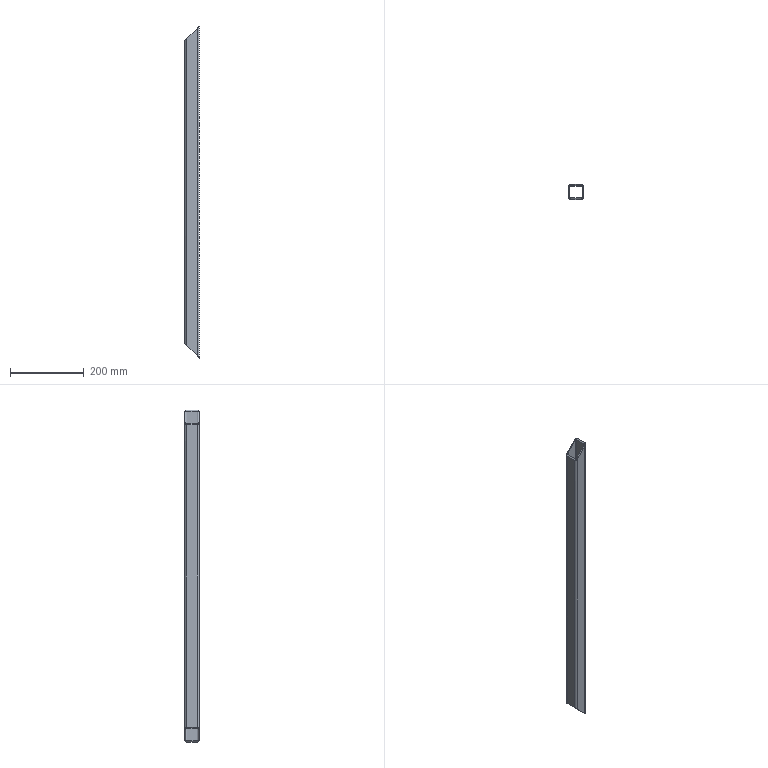Part | SolidWorks | features SavedExtBody 1 | 1 solid | 18 faces | box 40 x 40 x 900 mm | volume 382416 mm3 | plane 10 | cylinder 8 | commonest cylinder face diameters 6.4 x4 12.8 x4
STEP:
#1=CARTESIAN_POINT('',(13.6,440.,-443.6));
#2=VERTEX_POINT('',#1);
#3=CARTESIAN_POINT('',(20.,433.6,-450.));
#4=VERTEX_POINT('',#3);
#5=CARTESIAN_POINT('',(13.6,440.,-443.6));
#6=CARTESIAN_POINT('',(17.349,440.,-447.349));
#7=CARTESIAN_POINT('',(20.,437.349,-450.));
#8=CARTESIAN_POINT('',(20.,433.6,-450.));
#9=(BOUNDED_CURVE()B_SPLINE_CURVE(3,(#5,#6,#7,#8),.UNSPECIFIED.,.F.,.F.)B_SPLINE_CURVE_WITH_KNOTS((4,4),(4.712,6.283),.UNSPECIFIED.)CURVE()GEOMETRIC_REPRESENTATION_ITEM()RATIONAL_B_SPLINE_CURVE((1.,0.8047,0.8047,1.))REPRESENTATION_ITEM(''));
#10=EDGE_CURVE('',#2,#4,#9,.T.);
#11=ORIENTED_EDGE('',*,*,#10,.F.);
#12=CARTESIAN_POINT('',(13.6,440.,443.6));
#13=VERTEX_POINT('',#12);
#14=CARTESIAN_POINT('',(13.6,440.,430.));
#15=DIRECTION('',(0.,0.,-1.));
#16=VECTOR('',#15,1000.);
#17=LINE('',#14,#16);
#18=EDGE_CURVE('',#13,#2,#17,.T.);
#19=ORIENTED_EDGE('',*,*,#18,.F.);
#20=CARTESIAN_POINT('',(20.,433.6,450.));
#21=VERTEX_POINT('',#20);
#22=CARTESIAN_POINT('',(20.,433.6,450.));
#23=CARTESIAN_POINT('',(20.,437.349,450.));
#24=CARTESIAN_POINT('',(17.349,440.,447.349));
#25=CARTESIAN_POINT('',(13.6,440.,443.6));
#26=(BOUNDED_CURVE()B_SPLINE_CURVE(3,(#22,#23,#24,#25),.UNSPECIFIED.,.F.,.F.)B_SPLINE_CURVE_WITH_KNOTS((4,4),(3.142,4.712),.UNSPECIFIED.)CURVE()GEOMETRIC_REPRESENTATION_ITEM()RATIONAL_B_SPLINE_CURVE((1.,0.8047,0.8047,1.))REPRESENTATION_ITEM(''));
#27=EDGE_CURVE('',#21,#13,#26,.T.);
#28=ORIENTED_EDGE('',*,*,#27,.F.);
#29=CARTESIAN_POINT('',(20.,433.6,430.));
#30=DIRECTION('',(0.,0.,-1.));
#31=VECTOR('',#30,1000.);
#32=LINE('',#29,#31);
#33=EDGE_CURVE('',#21,#4,#32,.T.);
#34=ORIENTED_EDGE('',*,*,#33,.T.);
#35=EDGE_LOOP('',(#11,#19,#28,#34));
#36=FACE_OUTER_BOUND('',#35,.T.);
#37=CARTESIAN_POINT('',(13.6,433.6,430.));
#38=DIRECTION('',(0.,0.,-1.));
#39=DIRECTION('',(0.,1.,0.));
#40=AXIS2_PLACEMENT_3D('',#37,#38,#39);
#41=CYLINDRICAL_SURFACE('',#40,6.4);
#42=ADVANCED_FACE('',(#36),#41,.T.);
#43=CARTESIAN_POINT('',(-13.6,440.,-416.4));
#44=VERTEX_POINT('',#43);
#45=CARTESIAN_POINT('',(-423.2,440.,-6.8));
#46=DIRECTION('',(0.7071,0.,-0.7071));
#47=VECTOR('',#46,1000.);
#48=LINE('',#45,#47);
#49=EDGE_CURVE('',#44,#2,#48,.T.);
#50=ORIENTED_EDGE('',*,*,#49,.F.);
#51=CARTESIAN_POINT('',(-13.6,440.,416.4));
#52=VERTEX_POINT('',#51);
#53=CARTESIAN_POINT('',(-13.6,440.,430.));
#54=DIRECTION('',(0.,0.,-1.));
#55=VECTOR('',#54,1000.);
#56=LINE('',#53,#55);
#57=EDGE_CURVE('',#52,#44,#56,.T.);
#58=ORIENTED_EDGE('',*,*,#57,.F.);
#59=CARTESIAN_POINT('',(6.8,440.,436.8));
#60=DIRECTION('',(-0.7071,0.,-0.7071));
#61=VECTOR('',#60,1000.);
#62=LINE('',#59,#61);
#63=EDGE_CURVE('',#13,#52,#62,.T.);
#64=ORIENTED_EDGE('',*,*,#63,.F.);
#65=ORIENTED_EDGE('',*,*,#18,.T.);
#66=EDGE_LOOP('',(#50,#58,#64,#65));
#67=FACE_OUTER_BOUND('',#66,.T.);
#68=CARTESIAN_POINT('',(13.6,440.,430.));
#69=DIRECTION('',(0.,-1.,0.));
#70=DIRECTION('',(0.,0.,-1.));
#71=AXIS2_PLACEMENT_3D('',#68,#69,#70);
#72=PLANE('',#71);
#73=ADVANCED_FACE('',(#67),#72,.F.);
#74=CARTESIAN_POINT('',(-20.,433.6,-410.));
#75=VERTEX_POINT('',#74);
#76=CARTESIAN_POINT('',(-20.,433.6,-410.));
#77=CARTESIAN_POINT('',(-20.,437.349,-410.));
#78=CARTESIAN_POINT('',(-17.349,440.,-412.651));
#79=CARTESIAN_POINT('',(-13.6,440.,-416.4));
#80=(BOUNDED_CURVE()B_SPLINE_CURVE(3,(#76,#77,#78,#79),.UNSPECIFIED.,.F.,.F.)B_SPLINE_CURVE_WITH_KNOTS((4,4),(3.142,4.712),.UNSPECIFIED.)CURVE()GEOMETRIC_REPRESENTATION_ITEM()RATIONAL_B_SPLINE_CURVE((1.,0.8047,0.8047,1.))REPRESENTATION_ITEM(''));
#81=EDGE_CURVE('',#75,#44,#80,.T.);
#82=ORIENTED_EDGE('',*,*,#81,.F.);
#83=CARTESIAN_POINT('',(-20.,433.6,410.));
#84=VERTEX_POINT('',#83);
#85=CARTESIAN_POINT('',(-20.,433.6,430.));
#86=DIRECTION('',(0.,0.,-1.));
#87=VECTOR('',#86,1000.);
#88=LINE('',#85,#87);
#89=EDGE_CURVE('',#84,#75,#88,.T.);
#90=ORIENTED_EDGE('',*,*,#89,.F.);
#91=CARTESIAN_POINT('',(-13.6,440.,416.4));
#92=CARTESIAN_POINT('',(-17.349,440.,412.651));
#93=CARTESIAN_POINT('',(-20.,437.349,410.));
#94=CARTESIAN_POINT('',(-20.,433.6,410.));
#95=(BOUNDED_CURVE()B_SPLINE_CURVE(3,(#91,#92,#93,#94),.UNSPECIFIED.,.F.,.F.)B_SPLINE_CURVE_WITH_KNOTS((4,4),(4.712,6.283),.UNSPECIFIED.)CURVE()GEOMETRIC_REPRESENTATION_ITEM()RATIONAL_B_SPLINE_CURVE((1.,0.8047,0.8047,1.))REPRESENTATION_ITEM(''));
#96=EDGE_CURVE('',#52,#84,#95,.T.);
#97=ORIENTED_EDGE('',*,*,#96,.F.);
#98=ORIENTED_EDGE('',*,*,#57,.T.);
#99=EDGE_LOOP('',(#82,#90,#97,#98));
#100=FACE_OUTER_BOUND('',#99,.T.);
#101=CARTESIAN_POINT('',(-13.6,433.6,430.));
#102=DIRECTION('',(0.,0.,-1.));
#103=DIRECTION('',(0.,1.,0.));
#104=AXIS2_PLACEMENT_3D('',#101,#102,#103);
#105=CYLINDRICAL_SURFACE('',#104,6.4);
#106=ADVANCED_FACE('',(#100),#105,.T.);
#107=CARTESIAN_POINT('',(-20.,406.4,-410.));
#108=VERTEX_POINT('',#107);
#109=CARTESIAN_POINT('',(-20.,406.4,-410.));
#110=DIRECTION('',(0.,1.,0.));
#111=VECTOR('',#110,1000.);
#112=LINE('',#109,#111);
#113=EDGE_CURVE('',#108,#75,#112,.T.);
#114=ORIENTED_EDGE('',*,*,#113,.F.);
#115=CARTESIAN_POINT('',(-20.,406.4,410.));
#116=VERTEX_POINT('',#115);
#117=CARTESIAN_POINT('',(-20.,406.4,430.));
#118=DIRECTION('',(0.,0.,-1.));
#119=VECTOR('',#118,1000.);
#120=LINE('',#117,#119);
#121=EDGE_CURVE('',#116,#108,#120,.T.);
#122=ORIENTED_EDGE('',*,*,#121,.F.);
#123=CARTESIAN_POINT('',(-20.,406.4,410.));
#124=DIRECTION('',(0.,-1.,0.));
#125=VECTOR('',#124,1000.);
#126=LINE('',#123,#125);
#127=EDGE_CURVE('',#84,#116,#126,.T.);
#128=ORIENTED_EDGE('',*,*,#127,.F.);
#129=ORIENTED_EDGE('',*,*,#89,.T.);
#130=EDGE_LOOP('',(#114,#122,#128,#129));
#131=FACE_OUTER_BOUND('',#130,.T.);
#132=CARTESIAN_POINT('',(-20.,406.4,430.));
#133=DIRECTION('',(1.,0.,0.));
#134=DIRECTION('',(0.,1.,0.));
#135=AXIS2_PLACEMENT_3D('',#132,#133,#134);
#136=PLANE('',#135);
#137=ADVANCED_FACE('',(#131),#136,.F.);
#138=CARTESIAN_POINT('',(-13.6,400.,-416.4));
#139=VERTEX_POINT('',#138);
#140=CARTESIAN_POINT('',(-13.6,400.,-416.4));
#141=CARTESIAN_POINT('',(-17.349,400.,-412.651));
#142=CARTESIAN_POINT('',(-20.,402.651,-410.));
#143=CARTESIAN_POINT('',(-20.,406.4,-410.));
#144=(BOUNDED_CURVE()B_SPLINE_CURVE(3,(#140,#141,#142,#143),.UNSPECIFIED.,.F.,.F.)B_SPLINE_CURVE_WITH_KNOTS((4,4),(1.571,3.142),.UNSPECIFIED.)CURVE()GEOMETRIC_REPRESENTATION_ITEM()RATIONAL_B_SPLINE_CURVE((1.,0.8047,0.8047,1.))REPRESENTATION_ITEM(''));
#145=EDGE_CURVE('',#139,#108,#144,.T.);
#146=ORIENTED_EDGE('',*,*,#145,.F.);
#147=CARTESIAN_POINT('',(-13.6,400.,416.4));
#148=VERTEX_POINT('',#147);
#149=CARTESIAN_POINT('',(-13.6,400.,430.));
#150=DIRECTION('',(0.,0.,-1.));
#151=VECTOR('',#150,1000.);
#152=LINE('',#149,#151);
#153=EDGE_CURVE('',#148,#139,#152,.T.);
#154=ORIENTED_EDGE('',*,*,#153,.F.);
#155=CARTESIAN_POINT('',(-20.,406.4,410.));
#156=CARTESIAN_POINT('',(-20.,402.651,410.));
#157=CARTESIAN_POINT('',(-17.349,400.,412.651));
#158=CARTESIAN_POINT('',(-13.6,400.,416.4));
#159=(BOUNDED_CURVE()B_SPLINE_CURVE(3,(#155,#156,#157,#158),.UNSPECIFIED.,.F.,.F.)B_SPLINE_CURVE_WITH_KNOTS((4,4),(0.,1.571),.UNSPECIFIED.)CURVE()GEOMETRIC_REPRESENTATION_ITEM()RATIONAL_B_SPLINE_CURVE((1.,0.8047,0.8047,1.))REPRESENTATION_ITEM(''));
#160=EDGE_CURVE('',#116,#148,#159,.T.);
#161=ORIENTED_EDGE('',*,*,#160,.F.);
#162=ORIENTED_EDGE('',*,*,#121,.T.);
#163=EDGE_LOOP('',(#146,#154,#161,#162));
#164=FACE_OUTER_BOUND('',#163,.T.);
#165=CARTESIAN_POINT('',(-13.6,406.4,430.));
#166=DIRECTION('',(0.,0.,-1.));
#167=DIRECTION('',(0.,1.,0.));
#168=AXIS2_PLACEMENT_3D('',#165,#166,#167);
#169=CYLINDRICAL_SURFACE('',#168,6.4);
#170=ADVANCED_FACE('',(#164),#169,.T.);
#171=CARTESIAN_POINT('',(13.6,400.,-443.6));
#172=VERTEX_POINT('',#171);
#173=CARTESIAN_POINT('',(-436.8,400.,6.8));
#174=DIRECTION('',(-0.7071,0.,0.7071));
#175=VECTOR('',#174,1000.);
#176=LINE('',#173,#175);
#177=EDGE_CURVE('',#172,#139,#176,.T.);
#178=ORIENTED_EDGE('',*,*,#177,.F.);
#179=CARTESIAN_POINT('',(13.6,400.,443.6));
#180=VERTEX_POINT('',#179);
#181=CARTESIAN_POINT('',(13.6,400.,430.));
#182=DIRECTION('',(0.,0.,-1.));
#183=VECTOR('',#182,1000.);
#184=LINE('',#181,#183);
#185=EDGE_CURVE('',#180,#172,#184,.T.);
#186=ORIENTED_EDGE('',*,*,#185,.F.);
#187=CARTESIAN_POINT('',(-6.8,400.,423.2));
#188=DIRECTION('',(0.7071,0.,0.7071));
#189=VECTOR('',#188,1000.);
#190=LINE('',#187,#189);
#191=EDGE_CURVE('',#148,#180,#190,.T.);
#192=ORIENTED_EDGE('',*,*,#191,.F.);
#193=ORIENTED_EDGE('',*,*,#153,.T.);
#194=EDGE_LOOP('',(#178,#186,#192,#193));
#195=FACE_OUTER_BOUND('',#194,.T.);
#196=CARTESIAN_POINT('',(-13.6,400.,430.));
#197=DIRECTION('',(0.,1.,0.));
#198=DIRECTION('',(-1.,0.,0.));
#199=AXIS2_PLACEMENT_3D('',#196,#197,#198);
#200=PLANE('',#199);
#201=ADVANCED_FACE('',(#195),#200,.F.);
#202=CARTESIAN_POINT('',(20.,406.4,-450.));
#203=VERTEX_POINT('',#202);
#204=CARTESIAN_POINT('',(20.,406.4,-450.));
#205=CARTESIAN_POINT('',(20.,402.651,-450.));
#206=CARTESIAN_POINT('',(17.349,400.,-447.349));
#207=CARTESIAN_POINT('',(13.6,400.,-443.6));
#208=(BOUNDED_CURVE()B_SPLINE_CURVE(3,(#204,#205,#206,#207),.UNSPECIFIED.,.F.,.F.)B_SPLINE_CURVE_WITH_KNOTS((4,4),(0.,1.571),.UNSPECIFIED.)CURVE()GEOMETRIC_REPRESENTATION_ITEM()RATIONAL_B_SPLINE_CURVE((1.,0.8047,0.8047,1.))REPRESENTATION_ITEM(''));
#209=EDGE_CURVE('',#203,#172,#208,.T.);
#210=ORIENTED_EDGE('',*,*,#209,.F.);
#211=CARTESIAN_POINT('',(20.,406.4,450.));
#212=VERTEX_POINT('',#211);
#213=CARTESIAN_POINT('',(20.,406.4,430.));
#214=DIRECTION('',(0.,0.,-1.));
#215=VECTOR('',#214,1000.);
#216=LINE('',#213,#215);
#217=EDGE_CURVE('',#212,#203,#216,.T.);
#218=ORIENTED_EDGE('',*,*,#217,.F.);
#219=CARTESIAN_POINT('',(13.6,400.,443.6));
#220=CARTESIAN_POINT('',(17.349,400.,447.349));
#221=CARTESIAN_POINT('',(20.,402.651,450.));
#222=CARTESIAN_POINT('',(20.,406.4,450.));
#223=(BOUNDED_CURVE()B_SPLINE_CURVE(3,(#219,#220,#221,#222),.UNSPECIFIED.,.F.,.F.)B_SPLINE_CURVE_WITH_KNOTS((4,4),(1.571,3.142),.UNSPECIFIED.)CURVE()GEOMETRIC_REPRESENTATION_ITEM()RATIONAL_B_SPLINE_CURVE((1.,0.8047,0.8047,1.))REPRESENTATION_ITEM(''));
#224=EDGE_CURVE('',#180,#212,#223,.T.);
#225=ORIENTED_EDGE('',*,*,#224,.F.);
#226=ORIENTED_EDGE('',*,*,#185,.T.);
#227=EDGE_LOOP('',(#210,#218,#225,#226));
#228=FACE_OUTER_BOUND('',#227,.T.);
#229=CARTESIAN_POINT('',(13.6,406.4,430.));
#230=DIRECTION('',(0.,0.,-1.));
#231=DIRECTION('',(0.,1.,0.));
#232=AXIS2_PLACEMENT_3D('',#229,#230,#231);
#233=CYLINDRICAL_SURFACE('',#232,6.4);
#234=ADVANCED_FACE('',(#228),#233,.T.);
#235=CARTESIAN_POINT('',(-16.8,433.6,413.2));
#236=VERTEX_POINT('',#235);
#237=CARTESIAN_POINT('',(-16.8,433.6,-413.2));
#238=VERTEX_POINT('',#237);
#239=CARTESIAN_POINT('',(-16.8,433.6,430.));
#240=DIRECTION('',(0.,0.,-1.));
#241=VECTOR('',#240,1000.);
#242=LINE('',#239,#241);
#243=EDGE_CURVE('',#236,#238,#242,.T.);
#244=ORIENTED_EDGE('',*,*,#243,.T.);
#245=CARTESIAN_POINT('',(-13.6,436.8,-416.4));
#246=VERTEX_POINT('',#245);
#247=CARTESIAN_POINT('',(-16.8,433.6,-413.2));
#248=CARTESIAN_POINT('',(-16.8,435.475,-413.2));
#249=CARTESIAN_POINT('',(-15.475,436.8,-414.525));
#250=CARTESIAN_POINT('',(-13.6,436.8,-416.4));
#251=(BOUNDED_CURVE()B_SPLINE_CURVE(3,(#247,#248,#249,#250),.UNSPECIFIED.,.F.,.F.)B_SPLINE_CURVE_WITH_KNOTS((4,4),(3.142,4.712),.UNSPECIFIED.)CURVE()GEOMETRIC_REPRESENTATION_ITEM()RATIONAL_B_SPLINE_CURVE((1.,0.8047,0.8047,1.))REPRESENTATION_ITEM(''));
#252=EDGE_CURVE('',#238,#246,#251,.T.);
#253=ORIENTED_EDGE('',*,*,#252,.T.);
#254=CARTESIAN_POINT('',(-13.6,436.8,416.4));
#255=VERTEX_POINT('',#254);
#256=CARTESIAN_POINT('',(-13.6,436.8,430.));
#257=DIRECTION('',(0.,0.,-1.));
#258=VECTOR('',#257,1000.);
#259=LINE('',#256,#258);
#260=EDGE_CURVE('',#255,#246,#259,.T.);
#261=ORIENTED_EDGE('',*,*,#260,.F.);
#262=CARTESIAN_POINT('',(-13.6,436.8,416.4));
#263=CARTESIAN_POINT('',(-15.475,436.8,414.525));
#264=CARTESIAN_POINT('',(-16.8,435.475,413.2));
#265=CARTESIAN_POINT('',(-16.8,433.6,413.2));
#266=(BOUNDED_CURVE()B_SPLINE_CURVE(3,(#262,#263,#264,#265),.UNSPECIFIED.,.F.,.F.)B_SPLINE_CURVE_WITH_KNOTS((4,4),(4.712,6.283),.UNSPECIFIED.)CURVE()GEOMETRIC_REPRESENTATION_ITEM()RATIONAL_B_SPLINE_CURVE((1.,0.8047,0.8047,1.))REPRESENTATION_ITEM(''));
#267=EDGE_CURVE('',#255,#236,#266,.T.);
#268=ORIENTED_EDGE('',*,*,#267,.T.);
#269=EDGE_LOOP('',(#244,#253,#261,#268));
#270=FACE_OUTER_BOUND('',#269,.T.);
#271=CARTESIAN_POINT('',(-13.6,433.6,430.));
#272=DIRECTION('',(0.,0.,-1.));
#273=DIRECTION('',(0.,1.,0.));
#274=AXIS2_PLACEMENT_3D('',#271,#272,#273);
#275=CYLINDRICAL_SURFACE('',#274,3.2);
#276=ADVANCED_FACE('',(#270),#275,.F.);
#277=ORIENTED_EDGE('',*,*,#260,.T.);
#278=CARTESIAN_POINT('',(13.6,436.8,-443.6));
#279=VERTEX_POINT('',#278);
#280=CARTESIAN_POINT('',(-423.2,436.8,-6.8));
#281=DIRECTION('',(0.7071,0.,-0.7071));
#282=VECTOR('',#281,1000.);
#283=LINE('',#280,#282);
#284=EDGE_CURVE('',#246,#279,#283,.T.);
#285=ORIENTED_EDGE('',*,*,#284,.T.);
#286=CARTESIAN_POINT('',(13.6,436.8,443.6));
#287=VERTEX_POINT('',#286);
#288=CARTESIAN_POINT('',(13.6,436.8,430.));
#289=DIRECTION('',(0.,0.,-1.));
#290=VECTOR('',#289,1000.);
#291=LINE('',#288,#290);
#292=EDGE_CURVE('',#287,#279,#291,.T.);
#293=ORIENTED_EDGE('',*,*,#292,.F.);
#294=CARTESIAN_POINT('',(6.8,436.8,436.8));
#295=DIRECTION('',(-0.7071,0.,-0.7071));
#296=VECTOR('',#295,1000.);
#297=LINE('',#294,#296);
#298=EDGE_CURVE('',#287,#255,#297,.T.);
#299=ORIENTED_EDGE('',*,*,#298,.T.);
#300=EDGE_LOOP('',(#277,#285,#293,#299));
#301=FACE_OUTER_BOUND('',#300,.T.);
#302=CARTESIAN_POINT('',(13.6,436.8,430.));
#303=DIRECTION('',(0.,-1.,0.));
#304=DIRECTION('',(0.,0.,-1.));
#305=AXIS2_PLACEMENT_3D('',#302,#303,#304);
#306=PLANE('',#305);
#307=ADVANCED_FACE('',(#301),#306,.T.);
#308=ORIENTED_EDGE('',*,*,#292,.T.);
#309=CARTESIAN_POINT('',(16.8,433.6,-446.8));
#310=VERTEX_POINT('',#309);
#311=CARTESIAN_POINT('',(13.6,436.8,-443.6));
#312=CARTESIAN_POINT('',(15.475,436.8,-445.475));
#313=CARTESIAN_POINT('',(16.8,435.475,-446.8));
#314=CARTESIAN_POINT('',(16.8,433.6,-446.8));
#315=(BOUNDED_CURVE()B_SPLINE_CURVE(3,(#311,#312,#313,#314),.UNSPECIFIED.,.F.,.F.)B_SPLINE_CURVE_WITH_KNOTS((4,4),(4.712,6.283),.UNSPECIFIED.)CURVE()GEOMETRIC_REPRESENTATION_ITEM()RATIONAL_B_SPLINE_CURVE((1.,0.8047,0.8047,1.))REPRESENTATION_ITEM(''));
#316=EDGE_CURVE('',#279,#310,#315,.T.);
#317=ORIENTED_EDGE('',*,*,#316,.T.);
#318=CARTESIAN_POINT('',(16.8,433.6,446.8));
#319=VERTEX_POINT('',#318);
#320=CARTESIAN_POINT('',(16.8,433.6,430.));
#321=DIRECTION('',(0.,0.,-1.));
#322=VECTOR('',#321,1000.);
#323=LINE('',#320,#322);
#324=EDGE_CURVE('',#319,#310,#323,.T.);
#325=ORIENTED_EDGE('',*,*,#324,.F.);
#326=CARTESIAN_POINT('',(16.8,433.6,446.8));
#327=CARTESIAN_POINT('',(16.8,435.475,446.8));
#328=CARTESIAN_POINT('',(15.475,436.8,445.475));
#329=CARTESIAN_POINT('',(13.6,436.8,443.6));
#330=(BOUNDED_CURVE()B_SPLINE_CURVE(3,(#326,#327,#328,#329),.UNSPECIFIED.,.F.,.F.)B_SPLINE_CURVE_WITH_KNOTS((4,4),(3.142,4.712),.UNSPECIFIED.)CURVE()GEOMETRIC_REPRESENTATION_ITEM()RATIONAL_B_SPLINE_CURVE((1.,0.8047,0.8047,1.))REPRESENTATION_ITEM(''));
#331=EDGE_CURVE('',#319,#287,#330,.T.);
#332=ORIENTED_EDGE('',*,*,#331,.T.);
#333=EDGE_LOOP('',(#308,#317,#325,#332));
#334=FACE_OUTER_BOUND('',#333,.T.);
#335=CARTESIAN_POINT('',(13.6,433.6,430.));
#336=DIRECTION('',(0.,0.,-1.));
#337=DIRECTION('',(0.,1.,0.));
#338=AXIS2_PLACEMENT_3D('',#335,#336,#337);
#339=CYLINDRICAL_SURFACE('',#338,3.2);
#340=ADVANCED_FACE('',(#334),#339,.F.);
#341=ORIENTED_EDGE('',*,*,#324,.T.);
#342=CARTESIAN_POINT('',(16.8,406.4,-446.8));
#343=VERTEX_POINT('',#342);
#344=CARTESIAN_POINT('',(16.8,433.6,-446.8));
#345=DIRECTION('',(0.,-1.,0.));
#346=VECTOR('',#345,1000.);
#347=LINE('',#344,#346);
#348=EDGE_CURVE('',#310,#343,#347,.T.);
#349=ORIENTED_EDGE('',*,*,#348,.T.);
#350=CARTESIAN_POINT('',(16.8,406.4,446.8));
#351=VERTEX_POINT('',#350);
#352=CARTESIAN_POINT('',(16.8,406.4,430.));
#353=DIRECTION('',(0.,0.,-1.));
#354=VECTOR('',#353,1000.);
#355=LINE('',#352,#354);
#356=EDGE_CURVE('',#351,#343,#355,.T.);
#357=ORIENTED_EDGE('',*,*,#356,.F.);
#358=CARTESIAN_POINT('',(16.8,433.6,446.8));
#359=DIRECTION('',(0.,1.,0.));
#360=VECTOR('',#359,1000.);
#361=LINE('',#358,#360);
#362=EDGE_CURVE('',#351,#319,#361,.T.);
#363=ORIENTED_EDGE('',*,*,#362,.T.);
#364=EDGE_LOOP('',(#341,#349,#357,#363));
#365=FACE_OUTER_BOUND('',#364,.T.);
#366=CARTESIAN_POINT('',(16.8,433.6,430.));
#367=DIRECTION('',(-1.,0.,0.));
#368=DIRECTION('',(0.,-1.,0.));
#369=AXIS2_PLACEMENT_3D('',#366,#367,#368);
#370=PLANE('',#369);
#371=ADVANCED_FACE('',(#365),#370,.T.);
#372=ORIENTED_EDGE('',*,*,#356,.T.);
#373=CARTESIAN_POINT('',(13.6,403.2,-443.6));
#374=VERTEX_POINT('',#373);
#375=CARTESIAN_POINT('',(16.8,406.4,-446.8));
#376=CARTESIAN_POINT('',(16.8,404.525,-446.8));
#377=CARTESIAN_POINT('',(15.475,403.2,-445.475));
#378=CARTESIAN_POINT('',(13.6,403.2,-443.6));
#379=(BOUNDED_CURVE()B_SPLINE_CURVE(3,(#375,#376,#377,#378),.UNSPECIFIED.,.F.,.F.)B_SPLINE_CURVE_WITH_KNOTS((4,4),(0.,1.571),.UNSPECIFIED.)CURVE()GEOMETRIC_REPRESENTATION_ITEM()RATIONAL_B_SPLINE_CURVE((1.,0.8047,0.8047,1.))REPRESENTATION_ITEM(''));
#380=EDGE_CURVE('',#343,#374,#379,.T.);
#381=ORIENTED_EDGE('',*,*,#380,.T.);
#382=CARTESIAN_POINT('',(13.6,403.2,443.6));
#383=VERTEX_POINT('',#382);
#384=CARTESIAN_POINT('',(13.6,403.2,430.));
#385=DIRECTION('',(0.,0.,-1.));
#386=VECTOR('',#385,1000.);
#387=LINE('',#384,#386);
#388=EDGE_CURVE('',#383,#374,#387,.T.);
#389=ORIENTED_EDGE('',*,*,#388,.F.);
#390=CARTESIAN_POINT('',(13.6,403.2,443.6));
#391=CARTESIAN_POINT('',(15.475,403.2,445.475));
#392=CARTESIAN_POINT('',(16.8,404.525,446.8));
#393=CARTESIAN_POINT('',(16.8,406.4,446.8));
#394=(BOUNDED_CURVE()B_SPLINE_CURVE(3,(#390,#391,#392,#393),.UNSPECIFIED.,.F.,.F.)B_SPLINE_CURVE_WITH_KNOTS((4,4),(1.571,3.142),.UNSPECIFIED.)CURVE()GEOMETRIC_REPRESENTATION_ITEM()RATIONAL_B_SPLINE_CURVE((1.,0.8047,0.8047,1.))REPRESENTATION_ITEM(''));
#395=EDGE_CURVE('',#383,#351,#394,.T.);
#396=ORIENTED_EDGE('',*,*,#395,.T.);
#397=EDGE_LOOP('',(#372,#381,#389,#396));
#398=FACE_OUTER_BOUND('',#397,.T.);
#399=CARTESIAN_POINT('',(13.6,406.4,430.));
#400=DIRECTION('',(0.,0.,-1.));
#401=DIRECTION('',(0.,1.,0.));
#402=AXIS2_PLACEMENT_3D('',#399,#400,#401);
#403=CYLINDRICAL_SURFACE('',#402,3.2);
#404=ADVANCED_FACE('',(#398),#403,.F.);
#405=ORIENTED_EDGE('',*,*,#388,.T.);
#406=CARTESIAN_POINT('',(-13.6,403.2,-416.4));
#407=VERTEX_POINT('',#406);
#408=CARTESIAN_POINT('',(-436.8,403.2,6.8));
#409=DIRECTION('',(-0.7071,0.,0.7071));
#410=VECTOR('',#409,1000.);
#411=LINE('',#408,#410);
#412=EDGE_CURVE('',#374,#407,#411,.T.);
#413=ORIENTED_EDGE('',*,*,#412,.T.);
#414=CARTESIAN_POINT('',(-13.6,403.2,416.4));
#415=VERTEX_POINT('',#414);
#416=CARTESIAN_POINT('',(-13.6,403.2,430.));
#417=DIRECTION('',(0.,0.,-1.));
#418=VECTOR('',#417,1000.);
#419=LINE('',#416,#418);
#420=EDGE_CURVE('',#415,#407,#419,.T.);
#421=ORIENTED_EDGE('',*,*,#420,.F.);
#422=CARTESIAN_POINT('',(-6.8,403.2,423.2));
#423=DIRECTION('',(0.7071,0.,0.7071));
#424=VECTOR('',#423,1000.);
#425=LINE('',#422,#424);
#426=EDGE_CURVE('',#415,#383,#425,.T.);
#427=ORIENTED_EDGE('',*,*,#426,.T.);
#428=EDGE_LOOP('',(#405,#413,#421,#427));
#429=FACE_OUTER_BOUND('',#428,.T.);
#430=CARTESIAN_POINT('',(-13.6,403.2,430.));
#431=DIRECTION('',(0.,1.,0.));
#432=DIRECTION('',(-1.,0.,0.));
#433=AXIS2_PLACEMENT_3D('',#430,#431,#432);
#434=PLANE('',#433);
#435=ADVANCED_FACE('',(#429),#434,.T.);
#436=ORIENTED_EDGE('',*,*,#420,.T.);
#437=CARTESIAN_POINT('',(-16.8,406.4,-413.2));
#438=VERTEX_POINT('',#437);
#439=CARTESIAN_POINT('',(-13.6,403.2,-416.4));
#440=CARTESIAN_POINT('',(-15.475,403.2,-414.525));
#441=CARTESIAN_POINT('',(-16.8,404.525,-413.2));
#442=CARTESIAN_POINT('',(-16.8,406.4,-413.2));
#443=(BOUNDED_CURVE()B_SPLINE_CURVE(3,(#439,#440,#441,#442),.UNSPECIFIED.,.F.,.F.)B_SPLINE_CURVE_WITH_KNOTS((4,4),(1.571,3.142),.UNSPECIFIED.)CURVE()GEOMETRIC_REPRESENTATION_ITEM()RATIONAL_B_SPLINE_CURVE((1.,0.8047,0.8047,1.))REPRESENTATION_ITEM(''));
#444=EDGE_CURVE('',#407,#438,#443,.T.);
#445=ORIENTED_EDGE('',*,*,#444,.T.);
#446=CARTESIAN_POINT('',(-16.8,406.4,413.2));
#447=VERTEX_POINT('',#446);
#448=CARTESIAN_POINT('',(-16.8,406.4,430.));
#449=DIRECTION('',(0.,0.,-1.));
#450=VECTOR('',#449,1000.);
#451=LINE('',#448,#450);
#452=EDGE_CURVE('',#447,#438,#451,.T.);
#453=ORIENTED_EDGE('',*,*,#452,.F.);
#454=CARTESIAN_POINT('',(-16.8,406.4,413.2));
#455=CARTESIAN_POINT('',(-16.8,404.525,413.2));
#456=CARTESIAN_POINT('',(-15.475,403.2,414.525));
#457=CARTESIAN_POINT('',(-13.6,403.2,416.4));
#458=(BOUNDED_CURVE()B_SPLINE_CURVE(3,(#454,#455,#456,#457),.UNSPECIFIED.,.F.,.F.)B_SPLINE_CURVE_WITH_KNOTS((4,4),(0.,1.571),.UNSPECIFIED.)CURVE()GEOMETRIC_REPRESENTATION_ITEM()RATIONAL_B_SPLINE_CURVE((1.,0.8047,0.8047,1.))REPRESENTATION_ITEM(''));
#459=EDGE_CURVE('',#447,#415,#458,.T.);
#460=ORIENTED_EDGE('',*,*,#459,.T.);
#461=EDGE_LOOP('',(#436,#445,#453,#460));
#462=FACE_OUTER_BOUND('',#461,.T.);
#463=CARTESIAN_POINT('',(-13.6,406.4,430.));
#464=DIRECTION('',(0.,0.,-1.));
#465=DIRECTION('',(0.,1.,0.));
#466=AXIS2_PLACEMENT_3D('',#463,#464,#465);
#467=CYLINDRICAL_SURFACE('',#466,3.2);
#468=ADVANCED_FACE('',(#462),#467,.F.);
#469=ORIENTED_EDGE('',*,*,#452,.T.);
#470=CARTESIAN_POINT('',(-16.8,406.4,-413.2));
#471=DIRECTION('',(0.,1.,0.));
#472=VECTOR('',#471,1000.);
#473=LINE('',#470,#472);
#474=EDGE_CURVE('',#438,#238,#473,.T.);
#475=ORIENTED_EDGE('',*,*,#474,.T.);
#476=ORIENTED_EDGE('',*,*,#243,.F.);
#477=CARTESIAN_POINT('',(-16.8,406.4,413.2));
#478=DIRECTION('',(0.,-1.,0.));
#479=VECTOR('',#478,1000.);
#480=LINE('',#477,#479);
#481=EDGE_CURVE('',#236,#447,#480,.T.);
#482=ORIENTED_EDGE('',*,*,#481,.T.);
#483=EDGE_LOOP('',(#469,#475,#476,#482));
#484=FACE_OUTER_BOUND('',#483,.T.);
#485=CARTESIAN_POINT('',(-16.8,406.4,430.));
#486=DIRECTION('',(1.,0.,0.));
#487=DIRECTION('',(0.,1.,0.));
#488=AXIS2_PLACEMENT_3D('',#485,#486,#487);
#489=PLANE('',#488);
#490=ADVANCED_FACE('',(#484),#489,.T.);
#491=CARTESIAN_POINT('',(20.,433.6,-450.));
#492=DIRECTION('',(0.,-1.,0.));
#493=VECTOR('',#492,1000.);
#494=LINE('',#491,#493);
#495=EDGE_CURVE('',#4,#203,#494,.T.);
#496=ORIENTED_EDGE('',*,*,#495,.F.);
#497=ORIENTED_EDGE('',*,*,#33,.F.);
#498=CARTESIAN_POINT('',(20.,433.6,450.));
#499=DIRECTION('',(0.,1.,0.));
#500=VECTOR('',#499,1000.);
#501=LINE('',#498,#500);
#502=EDGE_CURVE('',#212,#21,#501,.T.);
#503=ORIENTED_EDGE('',*,*,#502,.F.);
#504=ORIENTED_EDGE('',*,*,#217,.T.);
#505=EDGE_LOOP('',(#496,#497,#503,#504));
#506=FACE_OUTER_BOUND('',#505,.T.);
#507=CARTESIAN_POINT('',(20.,433.6,430.));
#508=DIRECTION('',(-1.,0.,0.));
#509=DIRECTION('',(0.,-1.,0.));
#510=AXIS2_PLACEMENT_3D('',#507,#508,#509);
#511=PLANE('',#510);
#512=ADVANCED_FACE('',(#506),#511,.F.);
#513=ORIENTED_EDGE('',*,*,#267,.F.);
#514=ORIENTED_EDGE('',*,*,#298,.F.);
#515=ORIENTED_EDGE('',*,*,#331,.F.);
#516=ORIENTED_EDGE('',*,*,#362,.F.);
#517=ORIENTED_EDGE('',*,*,#395,.F.);
#518=ORIENTED_EDGE('',*,*,#426,.F.);
#519=ORIENTED_EDGE('',*,*,#459,.F.);
#520=ORIENTED_EDGE('',*,*,#481,.F.);
#521=EDGE_LOOP('',(#513,#514,#515,#516,#517,#518,#519,#520));
#522=FACE_BOUND('',#521,.T.);
#523=ORIENTED_EDGE('',*,*,#502,.T.);
#524=ORIENTED_EDGE('',*,*,#27,.T.);
#525=ORIENTED_EDGE('',*,*,#63,.T.);
#526=ORIENTED_EDGE('',*,*,#96,.T.);
#527=ORIENTED_EDGE('',*,*,#127,.T.);
#528=ORIENTED_EDGE('',*,*,#160,.T.);
#529=ORIENTED_EDGE('',*,*,#191,.T.);
#530=ORIENTED_EDGE('',*,*,#224,.T.);
#531=EDGE_LOOP('',(#523,#524,#525,#526,#527,#528,#529,#530));
#532=FACE_OUTER_BOUND('',#531,.T.);
#533=CARTESIAN_POINT('',(0.,420.,430.));
#534=DIRECTION('',(-0.7071,0.,0.7071));
#535=DIRECTION('',(0.7071,0.,0.7071));
#536=AXIS2_PLACEMENT_3D('',#533,#534,#535);
#537=PLANE('',#536);
#538=ADVANCED_FACE('',(#522,#532),#537,.T.);
#539=ORIENTED_EDGE('',*,*,#252,.F.);
#540=ORIENTED_EDGE('',*,*,#474,.F.);
#541=ORIENTED_EDGE('',*,*,#444,.F.);
#542=ORIENTED_EDGE('',*,*,#412,.F.);
#543=ORIENTED_EDGE('',*,*,#380,.F.);
#544=ORIENTED_EDGE('',*,*,#348,.F.);
#545=ORIENTED_EDGE('',*,*,#316,.F.);
#546=ORIENTED_EDGE('',*,*,#284,.F.);
#547=EDGE_LOOP('',(#539,#540,#541,#542,#543,#544,#545,#546));
#548=FACE_BOUND('',#547,.T.);
#549=ORIENTED_EDGE('',*,*,#49,.T.);
#550=ORIENTED_EDGE('',*,*,#10,.T.);
#551=ORIENTED_EDGE('',*,*,#495,.T.);
#552=ORIENTED_EDGE('',*,*,#209,.T.);
#553=ORIENTED_EDGE('',*,*,#177,.T.);
#554=ORIENTED_EDGE('',*,*,#145,.T.);
#555=ORIENTED_EDGE('',*,*,#113,.T.);
#556=ORIENTED_EDGE('',*,*,#81,.T.);
#557=EDGE_LOOP('',(#549,#550,#551,#552,#553,#554,#555,#556));
#558=FACE_OUTER_BOUND('',#557,.T.);
#559=CARTESIAN_POINT('',(0.,420.,-430.));
#560=DIRECTION('',(-0.7071,0.,-0.7071));
#561=DIRECTION('',(-0.7071,0.,0.7071));
#562=AXIS2_PLACEMENT_3D('',#559,#560,#561);
#563=PLANE('',#562);
#564=ADVANCED_FACE('',(#548,#558),#563,.T.);
#565=CLOSED_SHELL('',(#42,#73,#106,#137,#170,#201,#234,#276,#307,#340,#371,#404,#435,#468,#490,#512,#538,#564));
#566=MANIFOLD_SOLID_BREP('',#565);
#567=CARTESIAN_POINT('',(0.,0.,0.));
#568=DIRECTION('',(0.,0.,1.));
#569=DIRECTION('',(1.,0.,0.));
#570=AXIS2_PLACEMENT_3D('',#567,#568,#569);
#571=(LENGTH_UNIT()NAMED_UNIT(*)SI_UNIT(.MILLI.,.METRE.));
#572=UNCERTAINTY_MEASURE_WITH_UNIT(LENGTH_MEASURE(0.00001),#571,'','');
#573=(NAMED_UNIT(*)PLANE_ANGLE_UNIT()SI_UNIT($,.RADIAN.));
#574=(NAMED_UNIT(*)SI_UNIT($,.STERADIAN.)SOLID_ANGLE_UNIT());
#575=(GEOMETRIC_REPRESENTATION_CONTEXT(3)GLOBAL_UNCERTAINTY_ASSIGNED_CONTEXT((#572))GLOBAL_UNIT_ASSIGNED_CONTEXT((#571,#573,#574))REPRESENTATION_CONTEXT('',''));
#576=ADVANCED_BREP_SHAPE_REPRESENTATION('',(#566,#570),#575);